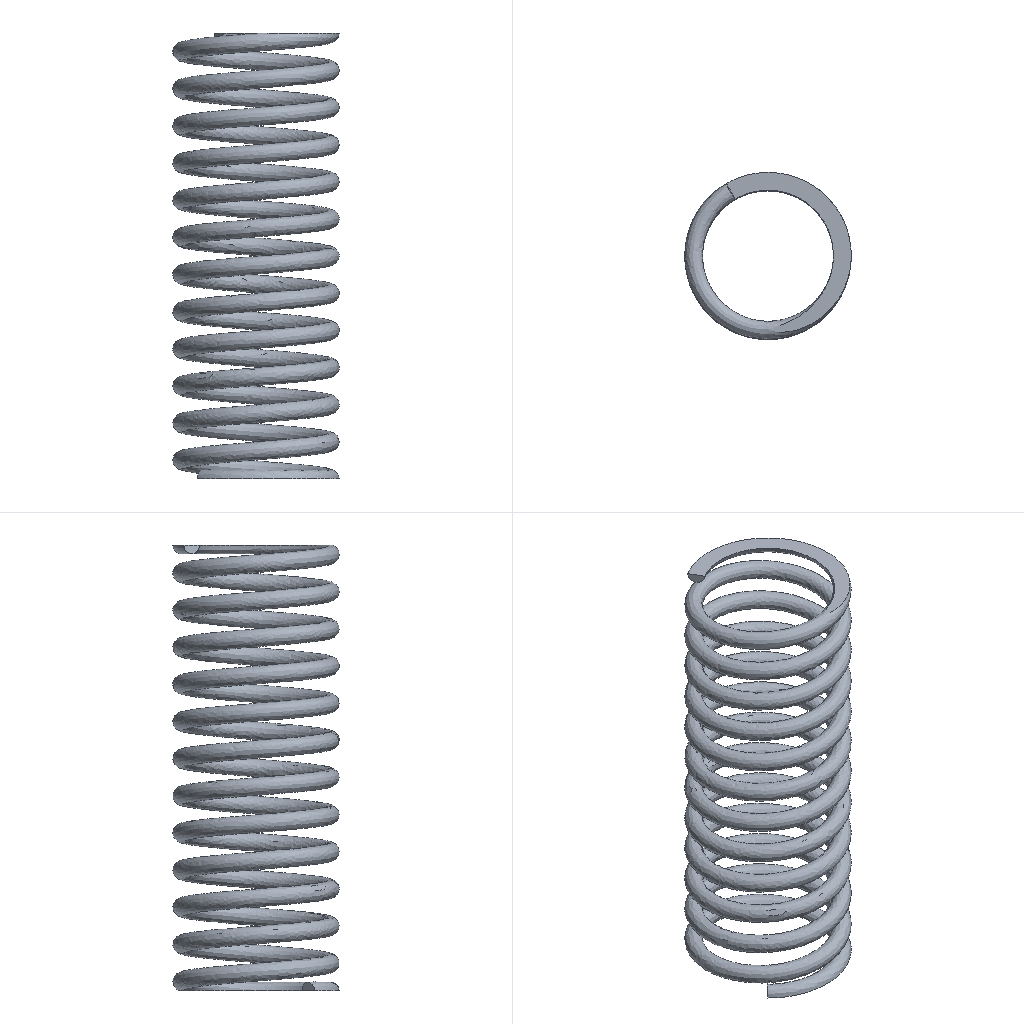Simulation study | ansys workbench
Ansys APDL input file, long lists of numbers shortened:
/batch
/config,noeldb,1     ! force off writing results to database
*get,_wallstrt,active,,time,wall
! ANSYS input file written by Workbench version 2023 R1
! File used for geometry attach:
/title,wbnew--__ (B5)
! ****** Begin Custom Load Command Snippet ******
/COM, ACT Extensions:
/COM,     LSDYNA, 2023.1
/COM,/COM,     ANSYSMotion, 2023.1
/COM,
! ****** End   Custom Load Command Snippet ******
*DIM,_wb_ProjectScratch_dir,string,248
_wb_ProjectScratch_dir(1) = ''
*DIM,_wb_SolverFiles_dir,string,248
_wb_SolverFiles_dir(1) = ''
*DIM,_wb_userfiles_dir,string,248
_wb_userfiles_dir(1) = ''
/com,--- Data in consistent MKS units. See Solving Units in the help system for more information.
/units,MKS
/nopr
/wb,file,start              !  signify a WB generated input file
/prep7
! Turn off shape checking because checks already performed inside WB mesher.
! See help system for more information.
SHPP,OFF,,NOWARN
/nolist
etcon,set             ! allow ANSYS to choose best KEYOP's for 180x elements, resets any applicable keyopt to MAPDL defaults
/com,*********** Nodes for the whole assembly ***********
nblock,3,,249216
(1i9,3e20.9e3)
        1    -4.403219008E-02    -4.923656381E-05     1.188127509E-02
! (226559 more lines like these left out)
-1
/wb,elem,start            !  set before creation of elements
/com,*********** Elements for Body 1 "Part12.8" ***********
et,1,187
eblock,19,solid,,139352
(19i9)
        1        1        1        1        0        0        0        0       10        0        1    22951    29275    34180    29278   184156   215198   184159   184157
! (278703 more lines like these left out)
-1
/wb,elem,end               !  done creating elements
/com,*********** Send User Defined Coordinate System(s) ***********
csys,0
toffst,273.15,  ! Temperature offset from absolute zero
/com,*********** Set Reference Temperature ***********
tref,22.
/wb,mat,start              !  starting to send materials
/com,*********** Send Materials ***********
MP,DENS,1,7850,	! kg m^-3
MP,EX,1,206000000000,	! Pa
MP,NUXY,1,0.3,
/wb,mat,end                !  done sending materials
!************************* Model Summary ********************
!Part12.8,	硅锰弹簧钢,	matid,	1
!************************* End Model Summary ********************
! get the diagonal of the bounding box. Needed later for other things
*get,_xmin,node,,mnloc,x
*get,_ymin,node,,mnloc,y
*get,_zmin,node,,mnloc,z
*get,_xmax,node,,mxloc,x
*get,_ymax,node,,mxloc,y
*get,_zmax,node,,mxloc,z
_ASMDIAG=(_xmax-_xmin)*(_xmax-_xmin)+(_ymax-_ymin)*(_ymax-_ymin)+(_zmax-_zmin)*(_zmax-_zmin)
_ASMDIAG=SQRT(_ASMDIAG)
/wb,contact,start          !  starting to send contact
/wb,contact,end            !  done creating contacts
/golist
/wb,load,start             !  starting to send loads
/gst,on,on
fini
*get,_numnode,node,0,count
*get,_numelem,elem,0,count
*get, _MAXELEMNUM, elem, 0, NUM, MAX
*get, _MAXNODENUM, node, 0, NUM, MAX
*get, _MAXELEMTYPE, etyp, 0, NUM, MAX
*get, _MAXREALCONST, rcon, 0, NUM, MAX
/go
/wb,load,end               !  done creating loads
/com,--- Number of total nodes = %_numnode%
/com,--- Number of contact elements = 0
/com,--- Number of spring elements = 0
/com,--- Number of bearing elements = 0
/com,--- Number of solid elements = 139352
/com,--- Number of condensed parts = 0
/com,--- Number of total elements = %_numelem%
*get,_wallbsol,active,,time,wall
/solu
antype,2                   ! modal analysis
_thickRatio=  1     ! Ratio of thick parts in the model
modopt,lanb,10
outres,erase
outres,all,none
outres,nsol,all
mxpand                    ! default expand in case of complex solution
dmpopt,esav,no
dmpopt,emat,no
dmpopt,full,no
! *********** WB SOLVE COMMAND ***********
! check interactive state
*get,ANSINTER_,active,,int
*if,ANSINTER_,ne,0,then
/eof
*endif
solve
/com *************** Write FE CONNECTORS *********
CEWRITE,file,ce,,INTE
*get,_nmodalsolproc,active,0,numcpu
fini
/nopr
*get,_numnode,node,0,count
*get,_numelem,elem,0,count
*get, _MAXELEMNUM, elem, 0, NUM, MAX
*get, _MAXNODENUM, node, 0, NUM, MAX,,,INTERNAL
*get, _MAXELEMTYPE, etyp, 0, NUM, MAX
*get, _MAXREALCONST, rcon, 0, NUM, MAX
*get,_NSOLTHREADS,active,0,ntfs
*get,_NSOLPROCESSES,active,0,npfs
/gopr
*get,_wallasol,active,,time,wall
/post1
/nopr
*dim,_direction,CHAR,6,1
_direction(1) = 'X'
_direction(2) = 'Y'
_direction(3) = 'Z'
_direction(4) = 'ROTX'
_direction(5) = 'ROTY'
_direction(6) = 'ROTZ'
*get,_lastLS,active,0,set,LSTP
*get,_beginset,active,0,set,nset,first,_lastLS
*get,_endset,active,0,set,nset,last,_lastLS
_nummodes = 0
*if,_endset,gt,0,then
_nummodes = _endset - _beginset + 1
*endif
*do,i_mode,1,_nummodes
   *do,j_component,1,6
			*get,PFACT_%i_mode%_%j_component%,MODE,%i_mode%,PFACT,,DIREC,_direction(%j_component%)
   *enddo
*enddo
*dim,_tmdirection,CHAR,6,1
_tmdirection(1) = 'X'
_tmdirection(2) = 'Y'
_tmdirection(3) = 'Z'
_tmdirection(4) = 'X'
_tmdirection(5) = 'Y'
_tmdirection(6) = 'Z'
*do,j_component,1,6
    *if,j_component,gt,3,then
        *get,TOTALMASS_%j_component%,ELEM,0,IOR,_tmdirection(%j_component%)
    *else
        *get,TOTALMASS_%j_component%,ELEM,0,MTOT,_tmdirection(%j_component%)
    *endif
*enddo
/gopr
xmlo,ENCODING,ISO-8859-1
xmlo,parm
/xml,parm,xml
fini
/gopr
*get,_walldone,active,,time,wall
_preptime=(_wallbsol-_wallstrt)*3600
_solvtime=(_wallasol-_wallbsol)*3600
_posttime=(_walldone-_wallasol)*3600
_totaltim=(_walldone-_wallstrt)*3600
*get,_dlbratio,active,0,solu,dlbr
*get,_combtime,active,0,solu,comb
*get,_ssmode,active,0,solu,ssmm
*get,_ndofs,active,0,solu,ndof
/fclean				!clean distributed files
/com,--- Total number of nodes = %_numnode%
/com,--- Total number of elements = %_numelem%
/com,--- Element load balance ratio = %_dlbratio%
/com,--- Time to combine distributed files = %_combtime%
/com,--- Sparse memory mode = %_ssmode%
/com,--- Number of DOF = %_ndofs%
/wb,file,end               ! done with WB generated input